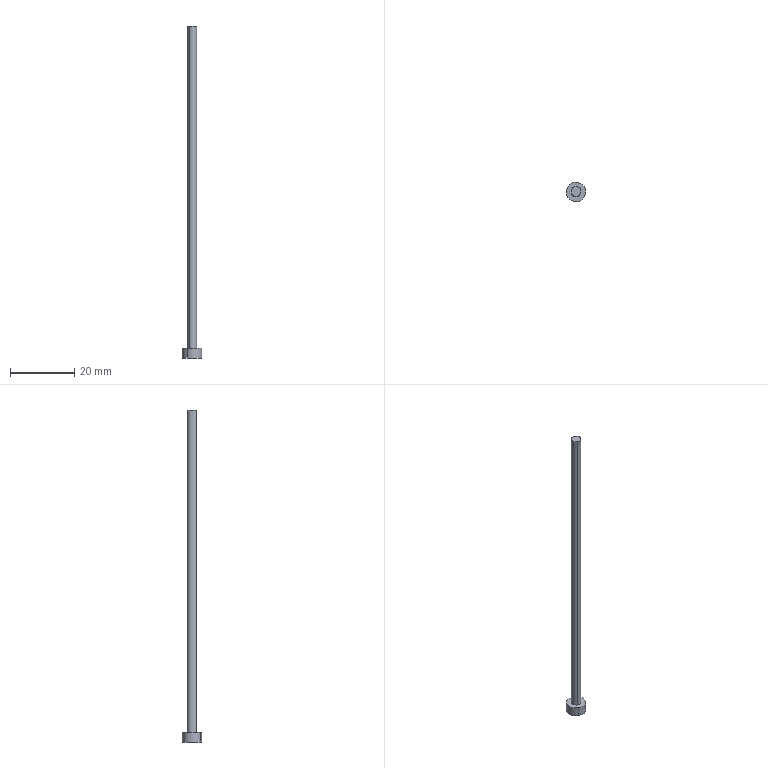Part | CATIA | 1 solid | 7 faces | box 6 x 6 x 103 mm | volume 791.681 mm3 | cylinder 4 | plane 3 | commonest cylinder face diameters 3 x2 6 x2
STEP:
#1=CARTESIAN_POINT('',(1.438,2.633,17.));
#2=VERTEX_POINT('',#1);
#3=CARTESIAN_POINT('',(-1.438,-2.633,17.));
#4=VERTEX_POINT('',#3);
#5=CARTESIAN_POINT('',(0.,0.,17.));
#6=DIRECTION('',(0.,0.,-1.));
#7=AXIS2_PLACEMENT_3D('',#5,#6,$);
#8=CIRCLE('',#7,3.);
#9=EDGE_CURVE('',#2,#4,#8,.T.);
#10=ORIENTED_EDGE('',*,*,#9,.F.);
#11=CARTESIAN_POINT('',(1.438,2.633,20.));
#12=VERTEX_POINT('',#11);
#13=CARTESIAN_POINT('',(1.438,2.633,18.5));
#14=DIRECTION('',(0.,0.,-1.));
#15=VECTOR('',#14,1.);
#16=LINE('',#13,#15);
#17=EDGE_CURVE('',#2,#12,#16,.F.);
#18=ORIENTED_EDGE('',*,*,#17,.T.);
#19=CARTESIAN_POINT('',(-1.438,-2.633,20.));
#20=VERTEX_POINT('',#19);
#21=CARTESIAN_POINT('',(0.,0.,20.));
#22=DIRECTION('',(0.,0.,-1.));
#23=AXIS2_PLACEMENT_3D('',#21,#22,$);
#24=CIRCLE('',#23,3.);
#25=EDGE_CURVE('',#12,#20,#24,.T.);
#26=ORIENTED_EDGE('',*,*,#25,.T.);
#27=CARTESIAN_POINT('',(-1.438,-2.633,18.5));
#28=DIRECTION('',(0.,0.,-1.));
#29=VECTOR('',#28,1.);
#30=LINE('',#27,#29);
#31=EDGE_CURVE('',#4,#20,#30,.F.);
#32=ORIENTED_EDGE('',*,*,#31,.F.);
#33=EDGE_LOOP('',(#10,#18,#26,#32));
#34=FACE_OUTER_BOUND('',#33,.T.);
#35=CARTESIAN_POINT('',(0.,0.,68.5));
#36=DIRECTION('',(0.,0.,-1.));
#37=DIRECTION('',(0.4794,0.8776,0.));
#38=AXIS2_PLACEMENT_3D('',#35,#36,#37);
#39=CYLINDRICAL_SURFACE('',#38,3.);
#40=ADVANCED_FACE('',(#34),#39,.T.);
#41=CARTESIAN_POINT('',(0.,0.,17.));
#42=DIRECTION('',(0.,0.,-1.));
#43=AXIS2_PLACEMENT_3D('',#41,#42,$);
#44=CIRCLE('',#43,3.);
#45=EDGE_CURVE('',#4,#2,#44,.T.);
#46=ORIENTED_EDGE('',*,*,#45,.F.);
#47=ORIENTED_EDGE('',*,*,#31,.T.);
#48=CARTESIAN_POINT('',(0.,0.,20.));
#49=DIRECTION('',(0.,0.,-1.));
#50=AXIS2_PLACEMENT_3D('',#48,#49,$);
#51=CIRCLE('',#50,3.);
#52=EDGE_CURVE('',#20,#12,#51,.T.);
#53=ORIENTED_EDGE('',*,*,#52,.T.);
#54=ORIENTED_EDGE('',*,*,#17,.F.);
#55=EDGE_LOOP('',(#46,#47,#53,#54));
#56=FACE_OUTER_BOUND('',#55,.T.);
#57=ADVANCED_FACE('',(#56),#39,.T.);
#58=CARTESIAN_POINT('',(0.7191,1.316,20.));
#59=VERTEX_POINT('',#58);
#60=CARTESIAN_POINT('',(-0.7191,-1.316,20.));
#61=VERTEX_POINT('',#60);
#62=CARTESIAN_POINT('',(0.,0.,20.));
#63=DIRECTION('',(0.,0.,-1.));
#64=AXIS2_PLACEMENT_3D('',#62,#63,$);
#65=CIRCLE('',#64,1.5);
#66=EDGE_CURVE('',#59,#61,#65,.T.);
#67=ORIENTED_EDGE('',*,*,#66,.F.);
#68=CARTESIAN_POINT('',(0.7191,1.316,120.));
#69=VERTEX_POINT('',#68);
#70=CARTESIAN_POINT('',(0.7191,1.316,70.));
#71=DIRECTION('',(0.,0.,-1.));
#72=VECTOR('',#71,1.);
#73=LINE('',#70,#72);
#74=EDGE_CURVE('',#59,#69,#73,.F.);
#75=ORIENTED_EDGE('',*,*,#74,.T.);
#76=CARTESIAN_POINT('',(-0.7191,-1.316,120.));
#77=VERTEX_POINT('',#76);
#78=CARTESIAN_POINT('',(0.,0.,120.));
#79=DIRECTION('',(0.,0.,-1.));
#80=AXIS2_PLACEMENT_3D('',#78,#79,$);
#81=CIRCLE('',#80,1.5);
#82=EDGE_CURVE('',#69,#77,#81,.T.);
#83=ORIENTED_EDGE('',*,*,#82,.T.);
#84=CARTESIAN_POINT('',(-0.7191,-1.316,70.));
#85=DIRECTION('',(0.,0.,-1.));
#86=VECTOR('',#85,1.);
#87=LINE('',#84,#86);
#88=EDGE_CURVE('',#61,#77,#87,.F.);
#89=ORIENTED_EDGE('',*,*,#88,.F.);
#90=EDGE_LOOP('',(#67,#75,#83,#89));
#91=FACE_OUTER_BOUND('',#90,.T.);
#92=CARTESIAN_POINT('',(0.,0.,68.5));
#93=DIRECTION('',(0.,0.,-1.));
#94=DIRECTION('',(0.4794,0.8776,0.));
#95=AXIS2_PLACEMENT_3D('',#92,#93,#94);
#96=CYLINDRICAL_SURFACE('',#95,1.5);
#97=ADVANCED_FACE('',(#91),#96,.T.);
#98=CARTESIAN_POINT('',(0.,0.,20.));
#99=DIRECTION('',(0.,0.,-1.));
#100=AXIS2_PLACEMENT_3D('',#98,#99,$);
#101=CIRCLE('',#100,1.5);
#102=EDGE_CURVE('',#61,#59,#101,.T.);
#103=ORIENTED_EDGE('',*,*,#102,.F.);
#104=ORIENTED_EDGE('',*,*,#88,.T.);
#105=CARTESIAN_POINT('',(0.,0.,120.));
#106=DIRECTION('',(0.,0.,-1.));
#107=AXIS2_PLACEMENT_3D('',#105,#106,$);
#108=CIRCLE('',#107,1.5);
#109=EDGE_CURVE('',#77,#69,#108,.T.);
#110=ORIENTED_EDGE('',*,*,#109,.T.);
#111=ORIENTED_EDGE('',*,*,#74,.F.);
#112=EDGE_LOOP('',(#103,#104,#110,#111));
#113=FACE_OUTER_BOUND('',#112,.T.);
#114=ADVANCED_FACE('',(#113),#96,.T.);
#115=ORIENTED_EDGE('',*,*,#9,.T.);
#116=ORIENTED_EDGE('',*,*,#45,.T.);
#117=EDGE_LOOP('',(#115,#116));
#118=FACE_OUTER_BOUND('',#117,.T.);
#119=CARTESIAN_POINT('',(0.,0.,17.));
#120=DIRECTION('',(0.,0.,-1.));
#121=DIRECTION('',(1.,0.,0.));
#122=AXIS2_PLACEMENT_3D('',#119,#120,#121);
#123=PLANE('',#122);
#124=ADVANCED_FACE('',(#118),#123,.T.);
#125=ORIENTED_EDGE('',*,*,#25,.F.);
#126=ORIENTED_EDGE('',*,*,#52,.F.);
#127=EDGE_LOOP('',(#125,#126));
#128=FACE_OUTER_BOUND('',#127,.T.);
#129=ORIENTED_EDGE('',*,*,#102,.T.);
#130=ORIENTED_EDGE('',*,*,#66,.T.);
#131=EDGE_LOOP('',(#129,#130));
#132=FACE_BOUND('',#131,.T.);
#133=CARTESIAN_POINT('',(0.,3.,20.));
#134=DIRECTION('',(0.,0.,-1.));
#135=DIRECTION('',(1.,0.,0.));
#136=AXIS2_PLACEMENT_3D('',#133,#134,#135);
#137=PLANE('',#136);
#138=ADVANCED_FACE('',(#128,#132),#137,.F.);
#139=ORIENTED_EDGE('',*,*,#82,.F.);
#140=ORIENTED_EDGE('',*,*,#109,.F.);
#141=EDGE_LOOP('',(#139,#140));
#142=FACE_OUTER_BOUND('',#141,.T.);
#143=CARTESIAN_POINT('',(0.,1.5,120.));
#144=DIRECTION('',(0.,0.,-1.));
#145=DIRECTION('',(1.,0.,0.));
#146=AXIS2_PLACEMENT_3D('',#143,#144,#145);
#147=PLANE('',#146);
#148=ADVANCED_FACE('',(#142),#147,.F.);
#149=CLOSED_SHELL('',(#40,#57,#97,#114,#124,#138,#148));
#150=MANIFOLD_SOLID_BREP('',#149);
#151=(LENGTH_UNIT()NAMED_UNIT(*)SI_UNIT(.MILLI.,.METRE.));
#152=UNCERTAINTY_MEASURE_WITH_UNIT(LENGTH_MEASURE(0.005),#151,'','');
#153=(NAMED_UNIT(*)PLANE_ANGLE_UNIT()SI_UNIT($,.RADIAN.));
#154=(NAMED_UNIT(*)SI_UNIT($,.STERADIAN.)SOLID_ANGLE_UNIT());
#155=(GEOMETRIC_REPRESENTATION_CONTEXT(3)GLOBAL_UNCERTAINTY_ASSIGNED_CONTEXT((#152))GLOBAL_UNIT_ASSIGNED_CONTEXT((#151,#153,#154))REPRESENTATION_CONTEXT('',''));
#156=ADVANCED_BREP_SHAPE_REPRESENTATION('',(#150),#155);